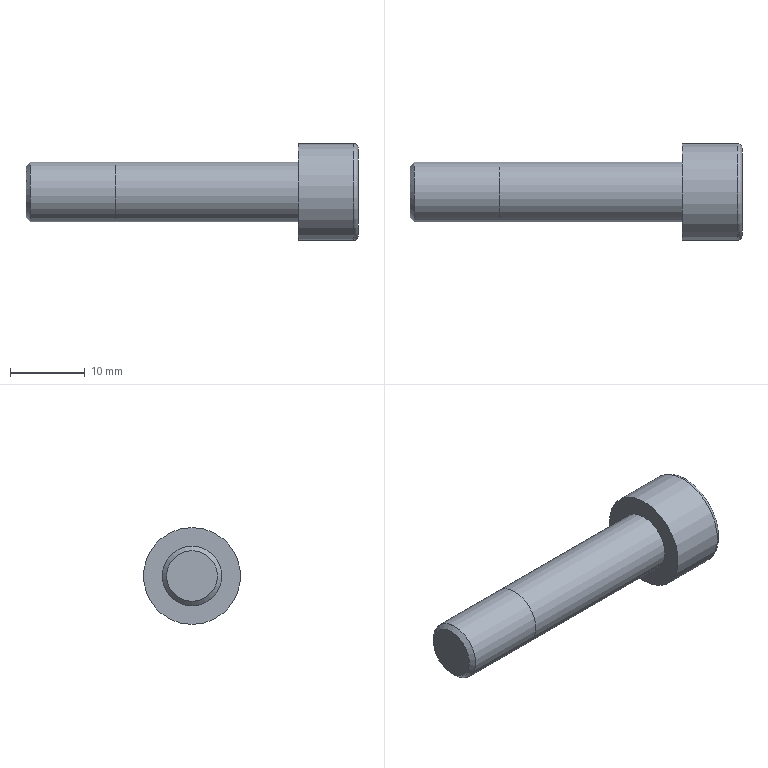Part | STEP file | solid 4 | 1 solid | 21 faces | box 44.5 x 13 x 13 mm | volume 2591 mm3 | plane 14 | cylinder 5 | torus 1 | cone 1 | commonest cylinder face diameters 6.8 x1 6.98 x1 7.99 x1 8 x1 13 x1